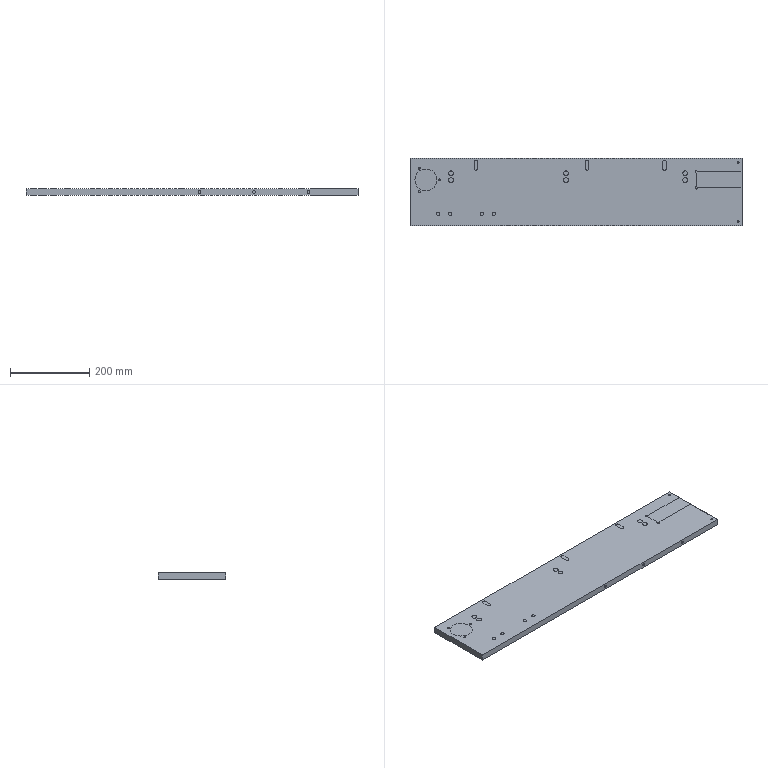Part | 2 solids | 100 faces | box 836 x 170 x 16 mm | volume 4410948 mm3 | cylinder 62 | plane 28 | cone 10 | commonest cylinder face diameters 5 x14 6.6 x12 12 x12 8.5 x8 6.8 x6 9 x6